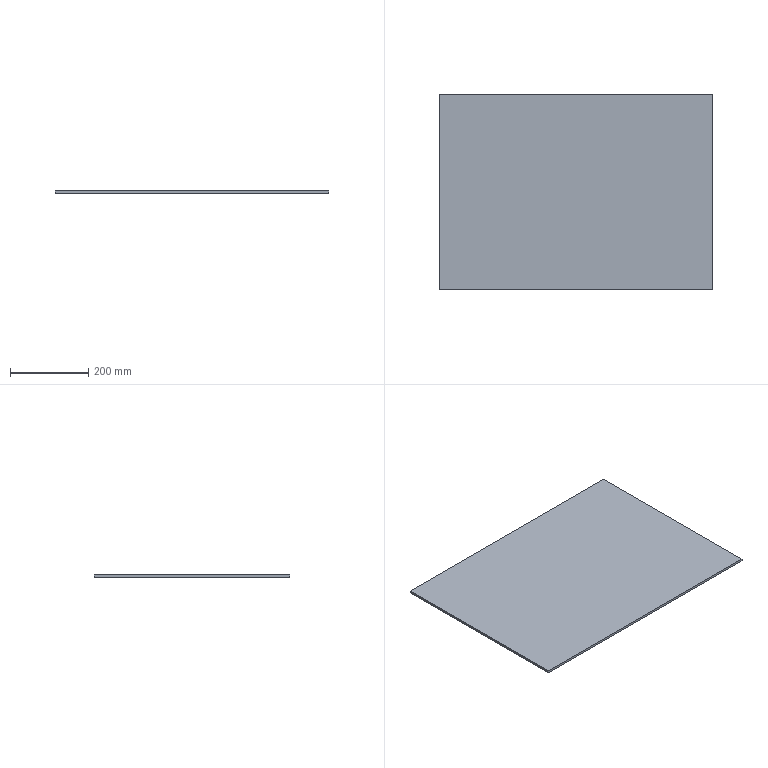Part | SolidWorks | features Extrusion 1 | 1 solid | 6 faces | box 700 x 500 x 6 mm | volume 2100000 mm3 | plane 6
STEP:
#1=CARTESIAN_POINT('',(350.,-250.,-3.));
#2=VERTEX_POINT('',#1);
#3=CARTESIAN_POINT('',(350.,250.,-3.));
#4=VERTEX_POINT('',#3);
#5=CARTESIAN_POINT('',(350.,-250.,-3.));
#6=DIRECTION('',(0.,1.,0.));
#7=VECTOR('',#6,1000.);
#8=LINE('',#5,#7);
#9=EDGE_CURVE('',#2,#4,#8,.T.);
#10=ORIENTED_EDGE('',*,*,#9,.T.);
#11=CARTESIAN_POINT('',(350.,250.,3.));
#12=VERTEX_POINT('',#11);
#13=CARTESIAN_POINT('',(350.,250.,3.));
#14=DIRECTION('',(0.,0.,-1.));
#15=VECTOR('',#14,1000.);
#16=LINE('',#13,#15);
#17=EDGE_CURVE('',#12,#4,#16,.T.);
#18=ORIENTED_EDGE('',*,*,#17,.F.);
#19=CARTESIAN_POINT('',(350.,-250.,3.));
#20=VERTEX_POINT('',#19);
#21=CARTESIAN_POINT('',(350.,-250.,3.));
#22=DIRECTION('',(0.,1.,0.));
#23=VECTOR('',#22,1000.);
#24=LINE('',#21,#23);
#25=EDGE_CURVE('',#20,#12,#24,.T.);
#26=ORIENTED_EDGE('',*,*,#25,.F.);
#27=CARTESIAN_POINT('',(350.,-250.,3.));
#28=DIRECTION('',(0.,0.,-1.));
#29=VECTOR('',#28,1000.);
#30=LINE('',#27,#29);
#31=EDGE_CURVE('',#20,#2,#30,.T.);
#32=ORIENTED_EDGE('',*,*,#31,.T.);
#33=EDGE_LOOP('',(#10,#18,#26,#32));
#34=FACE_OUTER_BOUND('',#33,.T.);
#35=CARTESIAN_POINT('',(350.,-250.,3.));
#36=DIRECTION('',(-1.,0.,0.));
#37=DIRECTION('',(0.,0.,1.));
#38=AXIS2_PLACEMENT_3D('',#35,#36,#37);
#39=PLANE('',#38);
#40=ADVANCED_FACE('',(#34),#39,.F.);
#41=CARTESIAN_POINT('',(-350.,250.,-3.));
#42=VERTEX_POINT('',#41);
#43=CARTESIAN_POINT('',(-350.,250.,-3.));
#44=DIRECTION('',(-1.,0.,0.));
#45=VECTOR('',#44,1000.);
#46=LINE('',#43,#45);
#47=EDGE_CURVE('',#4,#42,#46,.T.);
#48=ORIENTED_EDGE('',*,*,#47,.T.);
#49=CARTESIAN_POINT('',(-350.,250.,3.));
#50=VERTEX_POINT('',#49);
#51=CARTESIAN_POINT('',(-350.,250.,3.));
#52=DIRECTION('',(0.,0.,-1.));
#53=VECTOR('',#52,1000.);
#54=LINE('',#51,#53);
#55=EDGE_CURVE('',#50,#42,#54,.T.);
#56=ORIENTED_EDGE('',*,*,#55,.F.);
#57=CARTESIAN_POINT('',(-350.,250.,3.));
#58=DIRECTION('',(-1.,0.,0.));
#59=VECTOR('',#58,1000.);
#60=LINE('',#57,#59);
#61=EDGE_CURVE('',#12,#50,#60,.T.);
#62=ORIENTED_EDGE('',*,*,#61,.F.);
#63=ORIENTED_EDGE('',*,*,#17,.T.);
#64=EDGE_LOOP('',(#48,#56,#62,#63));
#65=FACE_OUTER_BOUND('',#64,.T.);
#66=CARTESIAN_POINT('',(-350.,250.,3.));
#67=DIRECTION('',(0.,-1.,0.));
#68=DIRECTION('',(0.,0.,-1.));
#69=AXIS2_PLACEMENT_3D('',#66,#67,#68);
#70=PLANE('',#69);
#71=ADVANCED_FACE('',(#65),#70,.F.);
#72=CARTESIAN_POINT('',(-350.,-250.,-3.));
#73=VERTEX_POINT('',#72);
#74=CARTESIAN_POINT('',(-350.,-250.,-3.));
#75=DIRECTION('',(0.,-1.,0.));
#76=VECTOR('',#75,1000.);
#77=LINE('',#74,#76);
#78=EDGE_CURVE('',#42,#73,#77,.T.);
#79=ORIENTED_EDGE('',*,*,#78,.T.);
#80=CARTESIAN_POINT('',(-350.,-250.,3.));
#81=VERTEX_POINT('',#80);
#82=CARTESIAN_POINT('',(-350.,-250.,3.));
#83=DIRECTION('',(0.,0.,-1.));
#84=VECTOR('',#83,1000.);
#85=LINE('',#82,#84);
#86=EDGE_CURVE('',#81,#73,#85,.T.);
#87=ORIENTED_EDGE('',*,*,#86,.F.);
#88=CARTESIAN_POINT('',(-350.,-250.,3.));
#89=DIRECTION('',(0.,-1.,0.));
#90=VECTOR('',#89,1000.);
#91=LINE('',#88,#90);
#92=EDGE_CURVE('',#50,#81,#91,.T.);
#93=ORIENTED_EDGE('',*,*,#92,.F.);
#94=ORIENTED_EDGE('',*,*,#55,.T.);
#95=EDGE_LOOP('',(#79,#87,#93,#94));
#96=FACE_OUTER_BOUND('',#95,.T.);
#97=CARTESIAN_POINT('',(-350.,-250.,3.));
#98=DIRECTION('',(1.,0.,0.));
#99=DIRECTION('',(0.,0.,-1.));
#100=AXIS2_PLACEMENT_3D('',#97,#98,#99);
#101=PLANE('',#100);
#102=ADVANCED_FACE('',(#96),#101,.F.);
#103=CARTESIAN_POINT('',(-350.,-250.,-3.));
#104=DIRECTION('',(1.,0.,0.));
#105=VECTOR('',#104,1000.);
#106=LINE('',#103,#105);
#107=EDGE_CURVE('',#73,#2,#106,.T.);
#108=ORIENTED_EDGE('',*,*,#107,.T.);
#109=ORIENTED_EDGE('',*,*,#31,.F.);
#110=CARTESIAN_POINT('',(-350.,-250.,3.));
#111=DIRECTION('',(1.,0.,0.));
#112=VECTOR('',#111,1000.);
#113=LINE('',#110,#112);
#114=EDGE_CURVE('',#81,#20,#113,.T.);
#115=ORIENTED_EDGE('',*,*,#114,.F.);
#116=ORIENTED_EDGE('',*,*,#86,.T.);
#117=EDGE_LOOP('',(#108,#109,#115,#116));
#118=FACE_OUTER_BOUND('',#117,.T.);
#119=CARTESIAN_POINT('',(-350.,-250.,3.));
#120=DIRECTION('',(0.,1.,0.));
#121=DIRECTION('',(0.,0.,1.));
#122=AXIS2_PLACEMENT_3D('',#119,#120,#121);
#123=PLANE('',#122);
#124=ADVANCED_FACE('',(#118),#123,.F.);
#125=ORIENTED_EDGE('',*,*,#25,.T.);
#126=ORIENTED_EDGE('',*,*,#61,.T.);
#127=ORIENTED_EDGE('',*,*,#92,.T.);
#128=ORIENTED_EDGE('',*,*,#114,.T.);
#129=EDGE_LOOP('',(#125,#126,#127,#128));
#130=FACE_OUTER_BOUND('',#129,.T.);
#131=CARTESIAN_POINT('',(0.,0.,3.));
#132=DIRECTION('',(0.,0.,-1.));
#133=DIRECTION('',(-1.,0.,0.));
#134=AXIS2_PLACEMENT_3D('',#131,#132,#133);
#135=PLANE('',#134);
#136=ADVANCED_FACE('',(#130),#135,.F.);
#137=ORIENTED_EDGE('',*,*,#9,.F.);
#138=ORIENTED_EDGE('',*,*,#107,.F.);
#139=ORIENTED_EDGE('',*,*,#78,.F.);
#140=ORIENTED_EDGE('',*,*,#47,.F.);
#141=EDGE_LOOP('',(#137,#138,#139,#140));
#142=FACE_OUTER_BOUND('',#141,.T.);
#143=CARTESIAN_POINT('',(0.,0.,-3.));
#144=DIRECTION('',(0.,0.,-1.));
#145=DIRECTION('',(-1.,0.,0.));
#146=AXIS2_PLACEMENT_3D('',#143,#144,#145);
#147=PLANE('',#146);
#148=ADVANCED_FACE('',(#142),#147,.T.);
#149=CLOSED_SHELL('',(#40,#71,#102,#124,#136,#148));
#150=MANIFOLD_SOLID_BREP('',#149);
#151=CARTESIAN_POINT('',(0.,0.,0.));
#152=DIRECTION('',(0.,0.,1.));
#153=DIRECTION('',(1.,0.,0.));
#154=AXIS2_PLACEMENT_3D('',#151,#152,#153);
#155=(LENGTH_UNIT()NAMED_UNIT(*)SI_UNIT(.MILLI.,.METRE.));
#156=UNCERTAINTY_MEASURE_WITH_UNIT(LENGTH_MEASURE(0.00001),#155,'','');
#157=(NAMED_UNIT(*)PLANE_ANGLE_UNIT()SI_UNIT($,.RADIAN.));
#158=(NAMED_UNIT(*)SI_UNIT($,.STERADIAN.)SOLID_ANGLE_UNIT());
#159=(GEOMETRIC_REPRESENTATION_CONTEXT(3)GLOBAL_UNCERTAINTY_ASSIGNED_CONTEXT((#156))GLOBAL_UNIT_ASSIGNED_CONTEXT((#155,#157,#158))REPRESENTATION_CONTEXT('',''));
#160=ADVANCED_BREP_SHAPE_REPRESENTATION('',(#150,#154),#159);